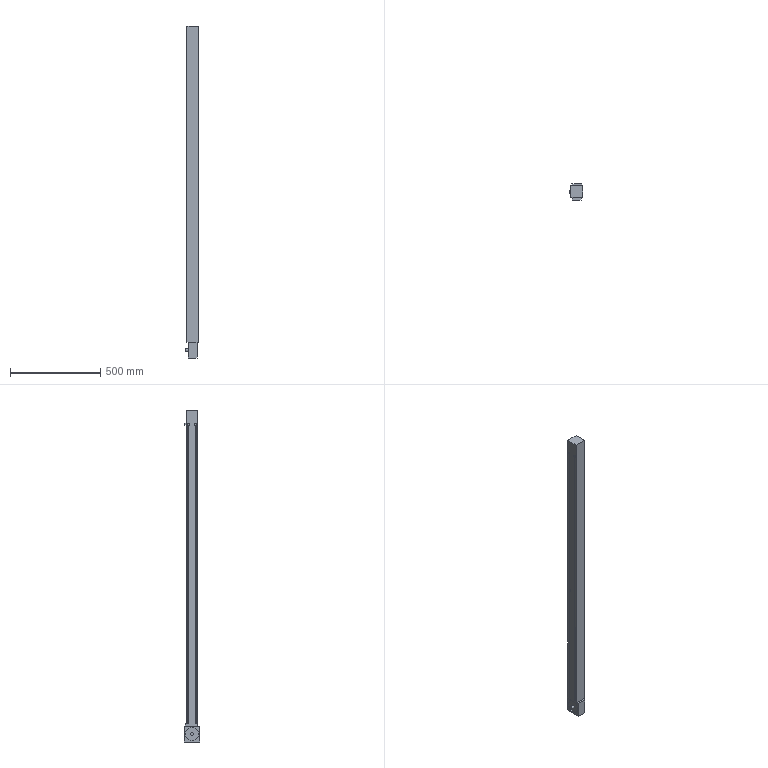Part | SolidWorks | features Boss 5, Cut 2, Extrusion 1, MirrorPattern 1 | 1 solid | 87 faces | box 72 x 88 x 1836 mm | volume 7220915 mm3 | plane 75 | cylinder 12 | commonest cylinder face diameters 8 x8 16 x2 73 x2